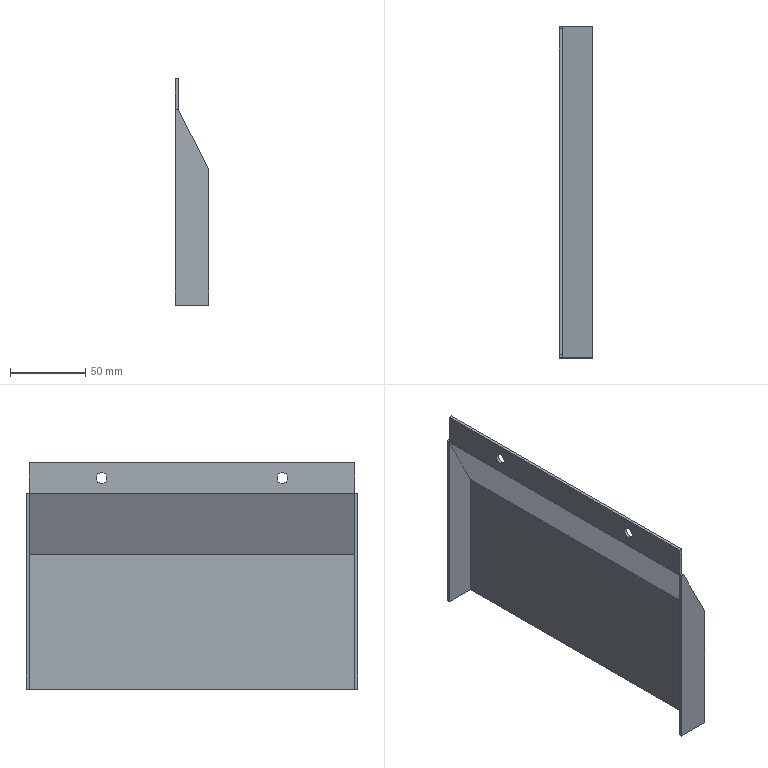Part | SolidWorks | features BaseBody 1 | 1 solid | 20 faces | box 22 x 220 x 150 mm | volume 76517 mm3 | plane 16 | cylinder 4 | commonest cylinder face diameters 7.2 x4
STEP:
#1=CARTESIAN_POINT('',(200.446,-4170.973,253.871));
#2=VERTEX_POINT('',#1);
#3=CARTESIAN_POINT('',(200.446,-4170.973,261.071));
#4=VERTEX_POINT('',#3);
#5=CARTESIAN_POINT('',(200.446,-4170.973,257.471));
#6=DIRECTION('',(-1.,0.,0.));
#7=DIRECTION('',(0.,0.,1.));
#8=AXIS2_PLACEMENT_3D('',#5,#6,#7);
#9=CIRCLE('',#8,3.6);
#10=EDGE_CURVE('',#2,#4,#9,.T.);
#11=ORIENTED_EDGE('',*,*,#10,.F.);
#12=CARTESIAN_POINT('',(198.446,-4170.973,253.871));
#13=VERTEX_POINT('',#12);
#14=CARTESIAN_POINT('',(199.279,-4170.973,253.871));
#15=DIRECTION('',(-1.,0.,0.));
#16=VECTOR('',#15,1000.);
#17=LINE('',#14,#16);
#18=EDGE_CURVE('',#2,#13,#17,.T.);
#19=ORIENTED_EDGE('',*,*,#18,.T.);
#20=CARTESIAN_POINT('',(198.446,-4170.973,261.071));
#21=VERTEX_POINT('',#20);
#22=CARTESIAN_POINT('',(198.446,-4170.973,257.471));
#23=DIRECTION('',(1.,0.,0.));
#24=DIRECTION('',(0.,0.,1.));
#25=AXIS2_PLACEMENT_3D('',#22,#23,#24);
#26=CIRCLE('',#25,3.6);
#27=EDGE_CURVE('',#21,#13,#26,.T.);
#28=ORIENTED_EDGE('',*,*,#27,.F.);
#29=CARTESIAN_POINT('',(199.279,-4170.973,261.071));
#30=DIRECTION('',(-1.,0.,0.));
#31=VECTOR('',#30,1000.);
#32=LINE('',#29,#31);
#33=EDGE_CURVE('',#4,#21,#32,.T.);
#34=ORIENTED_EDGE('',*,*,#33,.F.);
#35=EDGE_LOOP('',(#11,#19,#28,#34));
#36=FACE_OUTER_BOUND('',#35,.T.);
#37=CARTESIAN_POINT('',(199.279,-4170.973,257.471));
#38=DIRECTION('',(-1.,0.,0.));
#39=DIRECTION('',(0.,0.,1.));
#40=AXIS2_PLACEMENT_3D('',#37,#38,#39);
#41=CYLINDRICAL_SURFACE('',#40,3.6);
#42=ADVANCED_FACE('',(#36),#41,.F.);
#43=CARTESIAN_POINT('',(200.446,-4290.973,253.871));
#44=VERTEX_POINT('',#43);
#45=CARTESIAN_POINT('',(200.446,-4290.973,261.071));
#46=VERTEX_POINT('',#45);
#47=CARTESIAN_POINT('',(200.446,-4290.973,257.471));
#48=DIRECTION('',(-1.,0.,0.));
#49=DIRECTION('',(0.,0.,1.));
#50=AXIS2_PLACEMENT_3D('',#47,#48,#49);
#51=CIRCLE('',#50,3.6);
#52=EDGE_CURVE('',#44,#46,#51,.T.);
#53=ORIENTED_EDGE('',*,*,#52,.F.);
#54=CARTESIAN_POINT('',(198.446,-4290.973,253.871));
#55=VERTEX_POINT('',#54);
#56=CARTESIAN_POINT('',(199.279,-4290.973,253.871));
#57=DIRECTION('',(-1.,0.,0.));
#58=VECTOR('',#57,1000.);
#59=LINE('',#56,#58);
#60=EDGE_CURVE('',#44,#55,#59,.T.);
#61=ORIENTED_EDGE('',*,*,#60,.T.);
#62=CARTESIAN_POINT('',(198.446,-4290.973,261.071));
#63=VERTEX_POINT('',#62);
#64=CARTESIAN_POINT('',(198.446,-4290.973,257.471));
#65=DIRECTION('',(1.,0.,0.));
#66=DIRECTION('',(0.,0.,1.));
#67=AXIS2_PLACEMENT_3D('',#64,#65,#66);
#68=CIRCLE('',#67,3.6);
#69=EDGE_CURVE('',#63,#55,#68,.T.);
#70=ORIENTED_EDGE('',*,*,#69,.F.);
#71=CARTESIAN_POINT('',(199.279,-4290.973,261.071));
#72=DIRECTION('',(-1.,0.,0.));
#73=VECTOR('',#72,1000.);
#74=LINE('',#71,#73);
#75=EDGE_CURVE('',#46,#63,#74,.T.);
#76=ORIENTED_EDGE('',*,*,#75,.F.);
#77=EDGE_LOOP('',(#53,#61,#70,#76));
#78=FACE_OUTER_BOUND('',#77,.T.);
#79=CARTESIAN_POINT('',(199.279,-4290.973,257.471));
#80=DIRECTION('',(-1.,0.,0.));
#81=DIRECTION('',(0.,0.,1.));
#82=AXIS2_PLACEMENT_3D('',#79,#80,#81);
#83=CYLINDRICAL_SURFACE('',#82,3.6);
#84=ADVANCED_FACE('',(#78),#83,.F.);
#85=CARTESIAN_POINT('',(220.446,-4120.973,117.471));
#86=VERTEX_POINT('',#85);
#87=CARTESIAN_POINT('',(220.446,-4120.973,207.471));
#88=VERTEX_POINT('',#87);
#89=CARTESIAN_POINT('',(220.446,-4120.973,207.471));
#90=DIRECTION('',(0.,0.,1.));
#91=VECTOR('',#90,1000.);
#92=LINE('',#89,#91);
#93=EDGE_CURVE('',#86,#88,#92,.T.);
#94=ORIENTED_EDGE('',*,*,#93,.T.);
#95=CARTESIAN_POINT('',(220.446,-4340.973,207.471));
#96=VERTEX_POINT('',#95);
#97=CARTESIAN_POINT('',(220.446,-4140.973,207.471));
#98=DIRECTION('',(0.,-1.,0.));
#99=VECTOR('',#98,1000.);
#100=LINE('',#97,#99);
#101=EDGE_CURVE('',#88,#96,#100,.T.);
#102=ORIENTED_EDGE('',*,*,#101,.T.);
#103=CARTESIAN_POINT('',(220.446,-4340.973,117.471));
#104=VERTEX_POINT('',#103);
#105=CARTESIAN_POINT('',(220.446,-4340.973,207.471));
#106=DIRECTION('',(0.,0.,-1.));
#107=VECTOR('',#106,1000.);
#108=LINE('',#105,#107);
#109=EDGE_CURVE('',#96,#104,#108,.T.);
#110=ORIENTED_EDGE('',*,*,#109,.T.);
#111=CARTESIAN_POINT('',(220.446,-4140.973,117.471));
#112=DIRECTION('',(0.,1.,0.));
#113=VECTOR('',#112,1000.);
#114=LINE('',#111,#113);
#115=EDGE_CURVE('',#104,#86,#114,.T.);
#116=ORIENTED_EDGE('',*,*,#115,.T.);
#117=EDGE_LOOP('',(#94,#102,#110,#116));
#118=FACE_OUTER_BOUND('',#117,.T.);
#119=CARTESIAN_POINT('',(220.446,-4140.973,207.471));
#120=DIRECTION('',(1.,0.,0.));
#121=DIRECTION('',(0.,0.,-1.));
#122=AXIS2_PLACEMENT_3D('',#119,#120,#121);
#123=PLANE('',#122);
#124=ADVANCED_FACE('',(#118),#123,.T.);
#125=CARTESIAN_POINT('',(200.446,-4122.973,247.471));
#126=VERTEX_POINT('',#125);
#127=CARTESIAN_POINT('',(200.446,-4338.973,247.471));
#128=VERTEX_POINT('',#127);
#129=CARTESIAN_POINT('',(200.446,-4140.973,247.471));
#130=DIRECTION('',(0.,-1.,0.));
#131=VECTOR('',#130,1000.);
#132=LINE('',#129,#131);
#133=EDGE_CURVE('',#126,#128,#132,.T.);
#134=ORIENTED_EDGE('',*,*,#133,.T.);
#135=CARTESIAN_POINT('',(200.446,-4340.973,247.471));
#136=VERTEX_POINT('',#135);
#137=CARTESIAN_POINT('',(200.446,-4140.973,247.471));
#138=DIRECTION('',(0.,-1.,0.));
#139=VECTOR('',#138,1000.);
#140=LINE('',#137,#139);
#141=EDGE_CURVE('',#128,#136,#140,.T.);
#142=ORIENTED_EDGE('',*,*,#141,.T.);
#143=CARTESIAN_POINT('',(200.446,-4340.973,247.471));
#144=DIRECTION('',(0.4472,0.,-0.8944));
#145=VECTOR('',#144,1000.);
#146=LINE('',#143,#145);
#147=EDGE_CURVE('',#136,#96,#146,.T.);
#148=ORIENTED_EDGE('',*,*,#147,.T.);
#149=ORIENTED_EDGE('',*,*,#101,.F.);
#150=CARTESIAN_POINT('',(200.446,-4120.973,247.471));
#151=VERTEX_POINT('',#150);
#152=CARTESIAN_POINT('',(200.446,-4120.973,247.471));
#153=DIRECTION('',(-0.4472,0.,0.8944));
#154=VECTOR('',#153,1000.);
#155=LINE('',#152,#154);
#156=EDGE_CURVE('',#88,#151,#155,.T.);
#157=ORIENTED_EDGE('',*,*,#156,.T.);
#158=CARTESIAN_POINT('',(200.446,-4140.973,247.471));
#159=DIRECTION('',(0.,-1.,0.));
#160=VECTOR('',#159,1000.);
#161=LINE('',#158,#160);
#162=EDGE_CURVE('',#151,#126,#161,.T.);
#163=ORIENTED_EDGE('',*,*,#162,.T.);
#164=EDGE_LOOP('',(#134,#142,#148,#149,#157,#163));
#165=FACE_OUTER_BOUND('',#164,.T.);
#166=CARTESIAN_POINT('',(200.446,-4140.973,247.471));
#167=DIRECTION('',(0.8944,0.,0.4472));
#168=DIRECTION('',(0.4472,0.,-0.8944));
#169=AXIS2_PLACEMENT_3D('',#166,#167,#168);
#170=PLANE('',#169);
#171=ADVANCED_FACE('',(#165),#170,.T.);
#172=CARTESIAN_POINT('',(198.446,-4120.973,117.471));
#173=VERTEX_POINT('',#172);
#174=CARTESIAN_POINT('',(206.666,-4120.973,117.471));
#175=DIRECTION('',(-1.,0.,0.));
#176=VECTOR('',#175,1000.);
#177=LINE('',#174,#176);
#178=EDGE_CURVE('',#86,#173,#177,.T.);
#179=ORIENTED_EDGE('',*,*,#178,.T.);
#180=CARTESIAN_POINT('',(198.446,-4120.973,247.471));
#181=VERTEX_POINT('',#180);
#182=CARTESIAN_POINT('',(198.446,-4120.973,193.652));
#183=DIRECTION('',(0.,0.,1.));
#184=VECTOR('',#183,1000.);
#185=LINE('',#182,#184);
#186=EDGE_CURVE('',#173,#181,#185,.T.);
#187=ORIENTED_EDGE('',*,*,#186,.T.);
#188=CARTESIAN_POINT('',(206.666,-4120.973,247.471));
#189=DIRECTION('',(1.,0.,0.));
#190=VECTOR('',#189,1000.);
#191=LINE('',#188,#190);
#192=EDGE_CURVE('',#181,#151,#191,.T.);
#193=ORIENTED_EDGE('',*,*,#192,.T.);
#194=ORIENTED_EDGE('',*,*,#156,.F.);
#195=ORIENTED_EDGE('',*,*,#93,.F.);
#196=EDGE_LOOP('',(#179,#187,#193,#194,#195));
#197=FACE_OUTER_BOUND('',#196,.T.);
#198=CARTESIAN_POINT('',(206.666,-4120.973,193.652));
#199=DIRECTION('',(0.,1.,0.));
#200=DIRECTION('',(0.,0.,1.));
#201=AXIS2_PLACEMENT_3D('',#198,#199,#200);
#202=PLANE('',#201);
#203=ADVANCED_FACE('',(#197),#202,.T.);
#204=CARTESIAN_POINT('',(198.446,-4340.973,117.471));
#205=VERTEX_POINT('',#204);
#206=CARTESIAN_POINT('',(218.446,-4340.973,117.471));
#207=DIRECTION('',(-1.,0.,0.));
#208=VECTOR('',#207,1000.);
#209=LINE('',#206,#208);
#210=EDGE_CURVE('',#104,#205,#209,.T.);
#211=ORIENTED_EDGE('',*,*,#210,.T.);
#212=CARTESIAN_POINT('',(198.446,-4338.973,117.471));
#213=VERTEX_POINT('',#212);
#214=CARTESIAN_POINT('',(198.446,-4320.973,117.471));
#215=DIRECTION('',(0.,1.,0.));
#216=VECTOR('',#215,1000.);
#217=LINE('',#214,#216);
#218=EDGE_CURVE('',#205,#213,#217,.T.);
#219=ORIENTED_EDGE('',*,*,#218,.T.);
#220=CARTESIAN_POINT('',(218.446,-4338.973,117.471));
#221=VERTEX_POINT('',#220);
#222=CARTESIAN_POINT('',(218.446,-4338.973,117.471));
#223=DIRECTION('',(1.,0.,0.));
#224=VECTOR('',#223,1000.);
#225=LINE('',#222,#224);
#226=EDGE_CURVE('',#213,#221,#225,.T.);
#227=ORIENTED_EDGE('',*,*,#226,.T.);
#228=CARTESIAN_POINT('',(218.446,-4122.973,117.471));
#229=VERTEX_POINT('',#228);
#230=CARTESIAN_POINT('',(218.446,-4320.973,117.471));
#231=DIRECTION('',(0.,1.,0.));
#232=VECTOR('',#231,1000.);
#233=LINE('',#230,#232);
#234=EDGE_CURVE('',#221,#229,#233,.T.);
#235=ORIENTED_EDGE('',*,*,#234,.T.);
#236=CARTESIAN_POINT('',(198.446,-4122.973,117.471));
#237=VERTEX_POINT('',#236);
#238=CARTESIAN_POINT('',(218.446,-4122.973,117.471));
#239=DIRECTION('',(-1.,0.,0.));
#240=VECTOR('',#239,1000.);
#241=LINE('',#238,#240);
#242=EDGE_CURVE('',#229,#237,#241,.T.);
#243=ORIENTED_EDGE('',*,*,#242,.T.);
#244=CARTESIAN_POINT('',(198.446,-4320.973,117.471));
#245=DIRECTION('',(0.,1.,0.));
#246=VECTOR('',#245,1000.);
#247=LINE('',#244,#246);
#248=EDGE_CURVE('',#237,#173,#247,.T.);
#249=ORIENTED_EDGE('',*,*,#248,.T.);
#250=ORIENTED_EDGE('',*,*,#178,.F.);
#251=ORIENTED_EDGE('',*,*,#115,.F.);
#252=EDGE_LOOP('',(#211,#219,#227,#235,#243,#249,#250,#251));
#253=FACE_OUTER_BOUND('',#252,.T.);
#254=CARTESIAN_POINT('',(218.446,-4320.973,117.471));
#255=DIRECTION('',(0.,0.,-1.));
#256=DIRECTION('',(-1.,0.,0.));
#257=AXIS2_PLACEMENT_3D('',#254,#255,#256);
#258=PLANE('',#257);
#259=ADVANCED_FACE('',(#253),#258,.T.);
#260=ORIENTED_EDGE('',*,*,#109,.F.);
#261=ORIENTED_EDGE('',*,*,#147,.F.);
#262=CARTESIAN_POINT('',(198.446,-4340.973,247.471));
#263=VERTEX_POINT('',#262);
#264=CARTESIAN_POINT('',(206.666,-4340.973,247.471));
#265=DIRECTION('',(-1.,0.,0.));
#266=VECTOR('',#265,1000.);
#267=LINE('',#264,#266);
#268=EDGE_CURVE('',#136,#263,#267,.T.);
#269=ORIENTED_EDGE('',*,*,#268,.T.);
#270=CARTESIAN_POINT('',(198.446,-4340.973,193.652));
#271=DIRECTION('',(0.,0.,-1.));
#272=VECTOR('',#271,1000.);
#273=LINE('',#270,#272);
#274=EDGE_CURVE('',#263,#205,#273,.T.);
#275=ORIENTED_EDGE('',*,*,#274,.T.);
#276=ORIENTED_EDGE('',*,*,#210,.F.);
#277=EDGE_LOOP('',(#260,#261,#269,#275,#276));
#278=FACE_OUTER_BOUND('',#277,.T.);
#279=CARTESIAN_POINT('',(206.666,-4340.973,193.652));
#280=DIRECTION('',(0.,-1.,0.));
#281=DIRECTION('',(0.,0.,-1.));
#282=AXIS2_PLACEMENT_3D('',#279,#280,#281);
#283=PLANE('',#282);
#284=ADVANCED_FACE('',(#278),#283,.T.);
#285=CARTESIAN_POINT('',(198.446,-4338.973,247.471));
#286=VERTEX_POINT('',#285);
#287=CARTESIAN_POINT('',(213.457,-4338.973,247.471));
#288=DIRECTION('',(1.,0.,0.));
#289=VECTOR('',#288,1000.);
#290=LINE('',#287,#289);
#291=EDGE_CURVE('',#286,#128,#290,.T.);
#292=ORIENTED_EDGE('',*,*,#291,.F.);
#293=CARTESIAN_POINT('',(198.446,-4350.722,247.471));
#294=DIRECTION('',(0.,1.,0.));
#295=VECTOR('',#294,1000.);
#296=LINE('',#293,#295);
#297=EDGE_CURVE('',#263,#286,#296,.T.);
#298=ORIENTED_EDGE('',*,*,#297,.F.);
#299=ORIENTED_EDGE('',*,*,#268,.F.);
#300=ORIENTED_EDGE('',*,*,#141,.F.);
#301=EDGE_LOOP('',(#292,#298,#299,#300));
#302=FACE_OUTER_BOUND('',#301,.T.);
#303=CARTESIAN_POINT('',(213.457,-4350.722,247.471));
#304=DIRECTION('',(0.,0.,-1.));
#305=DIRECTION('',(-1.,0.,0.));
#306=AXIS2_PLACEMENT_3D('',#303,#304,#305);
#307=PLANE('',#306);
#308=ADVANCED_FACE('',(#302),#307,.F.);
#309=CARTESIAN_POINT('',(200.446,-4338.973,267.471));
#310=VERTEX_POINT('',#309);
#311=CARTESIAN_POINT('',(200.446,-4338.973,267.471));
#312=DIRECTION('',(0.,0.,-1.));
#313=VECTOR('',#312,1000.);
#314=LINE('',#311,#313);
#315=EDGE_CURVE('',#310,#128,#314,.T.);
#316=ORIENTED_EDGE('',*,*,#315,.T.);
#317=ORIENTED_EDGE('',*,*,#133,.F.);
#318=CARTESIAN_POINT('',(200.446,-4122.973,267.471));
#319=VERTEX_POINT('',#318);
#320=CARTESIAN_POINT('',(200.446,-4122.973,267.471));
#321=DIRECTION('',(0.,0.,1.));
#322=VECTOR('',#321,1000.);
#323=LINE('',#320,#322);
#324=EDGE_CURVE('',#126,#319,#323,.T.);
#325=ORIENTED_EDGE('',*,*,#324,.T.);
#326=CARTESIAN_POINT('',(200.446,-4140.973,267.471));
#327=DIRECTION('',(0.,-1.,0.));
#328=VECTOR('',#327,1000.);
#329=LINE('',#326,#328);
#330=EDGE_CURVE('',#319,#310,#329,.T.);
#331=ORIENTED_EDGE('',*,*,#330,.T.);
#332=EDGE_LOOP('',(#316,#317,#325,#331));
#333=FACE_OUTER_BOUND('',#332,.T.);
#334=CARTESIAN_POINT('',(200.446,-4170.973,257.471));
#335=DIRECTION('',(-1.,0.,0.));
#336=DIRECTION('',(0.,0.,1.));
#337=AXIS2_PLACEMENT_3D('',#334,#335,#336);
#338=CIRCLE('',#337,3.6);
#339=EDGE_CURVE('',#4,#2,#338,.T.);
#340=ORIENTED_EDGE('',*,*,#339,.T.);
#341=ORIENTED_EDGE('',*,*,#10,.T.);
#342=EDGE_LOOP('',(#340,#341));
#343=FACE_BOUND('',#342,.T.);
#344=CARTESIAN_POINT('',(200.446,-4290.973,257.471));
#345=DIRECTION('',(-1.,0.,0.));
#346=DIRECTION('',(0.,0.,1.));
#347=AXIS2_PLACEMENT_3D('',#344,#345,#346);
#348=CIRCLE('',#347,3.6);
#349=EDGE_CURVE('',#46,#44,#348,.T.);
#350=ORIENTED_EDGE('',*,*,#349,.T.);
#351=ORIENTED_EDGE('',*,*,#52,.T.);
#352=EDGE_LOOP('',(#350,#351));
#353=FACE_BOUND('',#352,.T.);
#354=CARTESIAN_POINT('',(200.446,-4140.973,267.471));
#355=DIRECTION('',(1.,0.,0.));
#356=DIRECTION('',(0.,0.,-1.));
#357=AXIS2_PLACEMENT_3D('',#354,#355,#356);
#358=PLANE('',#357);
#359=ADVANCED_FACE('',(#333,#343,#353),#358,.T.);
#360=CARTESIAN_POINT('',(198.446,-4122.973,247.471));
#361=VERTEX_POINT('',#360);
#362=CARTESIAN_POINT('',(213.457,-4122.973,247.471));
#363=DIRECTION('',(-1.,0.,0.));
#364=VECTOR('',#363,1000.);
#365=LINE('',#362,#364);
#366=EDGE_CURVE('',#126,#361,#365,.T.);
#367=ORIENTED_EDGE('',*,*,#366,.F.);
#368=ORIENTED_EDGE('',*,*,#162,.F.);
#369=ORIENTED_EDGE('',*,*,#192,.F.);
#370=CARTESIAN_POINT('',(198.446,-4111.225,247.471));
#371=DIRECTION('',(0.,1.,0.));
#372=VECTOR('',#371,1000.);
#373=LINE('',#370,#372);
#374=EDGE_CURVE('',#361,#181,#373,.T.);
#375=ORIENTED_EDGE('',*,*,#374,.F.);
#376=EDGE_LOOP('',(#367,#368,#369,#375));
#377=FACE_OUTER_BOUND('',#376,.T.);
#378=CARTESIAN_POINT('',(213.457,-4111.225,247.471));
#379=DIRECTION('',(0.,0.,-1.));
#380=DIRECTION('',(-1.,0.,0.));
#381=AXIS2_PLACEMENT_3D('',#378,#379,#380);
#382=PLANE('',#381);
#383=ADVANCED_FACE('',(#377),#382,.F.);
#384=CARTESIAN_POINT('',(198.446,-4338.973,267.471));
#385=VERTEX_POINT('',#384);
#386=CARTESIAN_POINT('',(198.446,-4122.973,267.471));
#387=VERTEX_POINT('',#386);
#388=CARTESIAN_POINT('',(198.446,-4280.973,267.471));
#389=DIRECTION('',(0.,1.,0.));
#390=VECTOR('',#389,1000.);
#391=LINE('',#388,#390);
#392=EDGE_CURVE('',#385,#387,#391,.T.);
#393=ORIENTED_EDGE('',*,*,#392,.T.);
#394=CARTESIAN_POINT('',(198.446,-4122.973,147.471));
#395=DIRECTION('',(0.,0.,-1.));
#396=VECTOR('',#395,1000.);
#397=LINE('',#394,#396);
#398=EDGE_CURVE('',#387,#361,#397,.T.);
#399=ORIENTED_EDGE('',*,*,#398,.T.);
#400=ORIENTED_EDGE('',*,*,#374,.T.);
#401=ORIENTED_EDGE('',*,*,#186,.F.);
#402=ORIENTED_EDGE('',*,*,#248,.F.);
#403=CARTESIAN_POINT('',(198.446,-4122.973,246.999));
#404=VERTEX_POINT('',#403);
#405=CARTESIAN_POINT('',(198.446,-4122.973,147.471));
#406=DIRECTION('',(0.,0.,1.));
#407=VECTOR('',#406,1000.);
#408=LINE('',#405,#407);
#409=EDGE_CURVE('',#237,#404,#408,.T.);
#410=ORIENTED_EDGE('',*,*,#409,.T.);
#411=CARTESIAN_POINT('',(198.446,-4338.973,246.999));
#412=VERTEX_POINT('',#411);
#413=CARTESIAN_POINT('',(198.446,-4280.973,246.999));
#414=DIRECTION('',(0.,-1.,0.));
#415=VECTOR('',#414,1000.);
#416=LINE('',#413,#415);
#417=EDGE_CURVE('',#404,#412,#416,.T.);
#418=ORIENTED_EDGE('',*,*,#417,.T.);
#419=CARTESIAN_POINT('',(198.446,-4338.973,147.471));
#420=DIRECTION('',(0.,0.,-1.));
#421=VECTOR('',#420,1000.);
#422=LINE('',#419,#421);
#423=EDGE_CURVE('',#412,#213,#422,.T.);
#424=ORIENTED_EDGE('',*,*,#423,.T.);
#425=ORIENTED_EDGE('',*,*,#218,.F.);
#426=ORIENTED_EDGE('',*,*,#274,.F.);
#427=ORIENTED_EDGE('',*,*,#297,.T.);
#428=CARTESIAN_POINT('',(198.446,-4338.973,147.471));
#429=DIRECTION('',(0.,0.,1.));
#430=VECTOR('',#429,1000.);
#431=LINE('',#428,#430);
#432=EDGE_CURVE('',#286,#385,#431,.T.);
#433=ORIENTED_EDGE('',*,*,#432,.T.);
#434=EDGE_LOOP('',(#393,#399,#400,#401,#402,#410,#418,#424,#425,#426,#427,#433));
#435=FACE_OUTER_BOUND('',#434,.T.);
#436=ORIENTED_EDGE('',*,*,#27,.T.);
#437=CARTESIAN_POINT('',(198.446,-4170.973,257.471));
#438=DIRECTION('',(1.,0.,0.));
#439=DIRECTION('',(0.,0.,1.));
#440=AXIS2_PLACEMENT_3D('',#437,#438,#439);
#441=CIRCLE('',#440,3.6);
#442=EDGE_CURVE('',#13,#21,#441,.T.);
#443=ORIENTED_EDGE('',*,*,#442,.T.);
#444=EDGE_LOOP('',(#436,#443));
#445=FACE_BOUND('',#444,.T.);
#446=ORIENTED_EDGE('',*,*,#69,.T.);
#447=CARTESIAN_POINT('',(198.446,-4290.973,257.471));
#448=DIRECTION('',(1.,0.,0.));
#449=DIRECTION('',(0.,0.,1.));
#450=AXIS2_PLACEMENT_3D('',#447,#448,#449);
#451=CIRCLE('',#450,3.6);
#452=EDGE_CURVE('',#55,#63,#451,.T.);
#453=ORIENTED_EDGE('',*,*,#452,.T.);
#454=EDGE_LOOP('',(#446,#453));
#455=FACE_BOUND('',#454,.T.);
#456=CARTESIAN_POINT('',(198.446,-4280.973,147.471));
#457=DIRECTION('',(-1.,0.,0.));
#458=DIRECTION('',(0.,0.,1.));
#459=AXIS2_PLACEMENT_3D('',#456,#457,#458);
#460=PLANE('',#459);
#461=ADVANCED_FACE('',(#435,#445,#455),#460,.T.);
#462=ORIENTED_EDGE('',*,*,#409,.F.);
#463=ORIENTED_EDGE('',*,*,#242,.F.);
#464=CARTESIAN_POINT('',(218.446,-4122.973,206.999));
#465=VERTEX_POINT('',#464);
#466=CARTESIAN_POINT('',(218.446,-4122.973,193.652));
#467=DIRECTION('',(0.,0.,-1.));
#468=VECTOR('',#467,1000.);
#469=LINE('',#466,#468);
#470=EDGE_CURVE('',#465,#229,#469,.T.);
#471=ORIENTED_EDGE('',*,*,#470,.F.);
#472=CARTESIAN_POINT('',(198.446,-4122.973,246.999));
#473=DIRECTION('',(0.4472,0.,-0.8944));
#474=VECTOR('',#473,1000.);
#475=LINE('',#472,#474);
#476=EDGE_CURVE('',#404,#465,#475,.T.);
#477=ORIENTED_EDGE('',*,*,#476,.F.);
#478=EDGE_LOOP('',(#462,#463,#471,#477));
#479=FACE_OUTER_BOUND('',#478,.T.);
#480=CARTESIAN_POINT('',(206.666,-4122.973,193.652));
#481=DIRECTION('',(0.,1.,0.));
#482=DIRECTION('',(0.,0.,1.));
#483=AXIS2_PLACEMENT_3D('',#480,#481,#482);
#484=PLANE('',#483);
#485=ADVANCED_FACE('',(#479),#484,.F.);
#486=ORIENTED_EDGE('',*,*,#470,.T.);
#487=ORIENTED_EDGE('',*,*,#234,.F.);
#488=CARTESIAN_POINT('',(218.446,-4338.973,206.999));
#489=VERTEX_POINT('',#488);
#490=CARTESIAN_POINT('',(218.446,-4338.973,117.471));
#491=DIRECTION('',(0.,0.,1.));
#492=VECTOR('',#491,1000.);
#493=LINE('',#490,#492);
#494=EDGE_CURVE('',#221,#489,#493,.T.);
#495=ORIENTED_EDGE('',*,*,#494,.T.);
#496=CARTESIAN_POINT('',(218.446,-4140.973,206.999));
#497=DIRECTION('',(0.,1.,0.));
#498=VECTOR('',#497,1000.);
#499=LINE('',#496,#498);
#500=EDGE_CURVE('',#489,#465,#499,.T.);
#501=ORIENTED_EDGE('',*,*,#500,.T.);
#502=EDGE_LOOP('',(#486,#487,#495,#501));
#503=FACE_OUTER_BOUND('',#502,.T.);
#504=CARTESIAN_POINT('',(218.446,-4140.973,117.471));
#505=DIRECTION('',(-1.,0.,0.));
#506=DIRECTION('',(0.,0.,1.));
#507=AXIS2_PLACEMENT_3D('',#504,#505,#506);
#508=PLANE('',#507);
#509=ADVANCED_FACE('',(#503),#508,.T.);
#510=ORIENTED_EDGE('',*,*,#494,.F.);
#511=ORIENTED_EDGE('',*,*,#226,.F.);
#512=ORIENTED_EDGE('',*,*,#423,.F.);
#513=CARTESIAN_POINT('',(218.446,-4338.973,206.999));
#514=DIRECTION('',(-0.4472,0.,0.8944));
#515=VECTOR('',#514,1000.);
#516=LINE('',#513,#515);
#517=EDGE_CURVE('',#489,#412,#516,.T.);
#518=ORIENTED_EDGE('',*,*,#517,.F.);
#519=EDGE_LOOP('',(#510,#511,#512,#518));
#520=FACE_OUTER_BOUND('',#519,.T.);
#521=CARTESIAN_POINT('',(206.666,-4338.973,193.652));
#522=DIRECTION('',(0.,-1.,0.));
#523=DIRECTION('',(0.,0.,-1.));
#524=AXIS2_PLACEMENT_3D('',#521,#522,#523);
#525=PLANE('',#524);
#526=ADVANCED_FACE('',(#520),#525,.F.);
#527=CARTESIAN_POINT('',(213.457,-4338.973,267.471));
#528=DIRECTION('',(1.,0.,0.));
#529=VECTOR('',#528,1000.);
#530=LINE('',#527,#529);
#531=EDGE_CURVE('',#385,#310,#530,.T.);
#532=ORIENTED_EDGE('',*,*,#531,.F.);
#533=ORIENTED_EDGE('',*,*,#432,.F.);
#534=ORIENTED_EDGE('',*,*,#291,.T.);
#535=ORIENTED_EDGE('',*,*,#315,.F.);
#536=EDGE_LOOP('',(#532,#533,#534,#535));
#537=FACE_OUTER_BOUND('',#536,.T.);
#538=CARTESIAN_POINT('',(213.457,-4338.973,247.471));
#539=DIRECTION('',(0.,1.,0.));
#540=DIRECTION('',(0.,0.,1.));
#541=AXIS2_PLACEMENT_3D('',#538,#539,#540);
#542=PLANE('',#541);
#543=ADVANCED_FACE('',(#537),#542,.F.);
#544=ORIENTED_EDGE('',*,*,#531,.T.);
#545=ORIENTED_EDGE('',*,*,#330,.F.);
#546=CARTESIAN_POINT('',(198.446,-4122.973,267.471));
#547=DIRECTION('',(-1.,0.,0.));
#548=VECTOR('',#547,1000.);
#549=LINE('',#546,#548);
#550=EDGE_CURVE('',#319,#387,#549,.T.);
#551=ORIENTED_EDGE('',*,*,#550,.T.);
#552=ORIENTED_EDGE('',*,*,#392,.F.);
#553=EDGE_LOOP('',(#544,#545,#551,#552));
#554=FACE_OUTER_BOUND('',#553,.T.);
#555=CARTESIAN_POINT('',(198.446,-4140.973,267.471));
#556=DIRECTION('',(0.,0.,1.));
#557=DIRECTION('',(1.,0.,0.));
#558=AXIS2_PLACEMENT_3D('',#555,#556,#557);
#559=PLANE('',#558);
#560=ADVANCED_FACE('',(#554),#559,.T.);
#561=ORIENTED_EDGE('',*,*,#550,.F.);
#562=ORIENTED_EDGE('',*,*,#324,.F.);
#563=ORIENTED_EDGE('',*,*,#366,.T.);
#564=ORIENTED_EDGE('',*,*,#398,.F.);
#565=EDGE_LOOP('',(#561,#562,#563,#564));
#566=FACE_OUTER_BOUND('',#565,.T.);
#567=CARTESIAN_POINT('',(213.457,-4122.973,247.471));
#568=DIRECTION('',(0.,-1.,0.));
#569=DIRECTION('',(0.,0.,-1.));
#570=AXIS2_PLACEMENT_3D('',#567,#568,#569);
#571=PLANE('',#570);
#572=ADVANCED_FACE('',(#566),#571,.F.);
#573=ORIENTED_EDGE('',*,*,#18,.F.);
#574=ORIENTED_EDGE('',*,*,#339,.F.);
#575=ORIENTED_EDGE('',*,*,#33,.T.);
#576=ORIENTED_EDGE('',*,*,#442,.F.);
#577=EDGE_LOOP('',(#573,#574,#575,#576));
#578=FACE_OUTER_BOUND('',#577,.T.);
#579=CARTESIAN_POINT('',(199.279,-4170.973,257.471));
#580=DIRECTION('',(-1.,0.,0.));
#581=DIRECTION('',(0.,0.,1.));
#582=AXIS2_PLACEMENT_3D('',#579,#580,#581);
#583=CYLINDRICAL_SURFACE('',#582,3.6);
#584=ADVANCED_FACE('',(#578),#583,.F.);
#585=ORIENTED_EDGE('',*,*,#60,.F.);
#586=ORIENTED_EDGE('',*,*,#349,.F.);
#587=ORIENTED_EDGE('',*,*,#75,.T.);
#588=ORIENTED_EDGE('',*,*,#452,.F.);
#589=EDGE_LOOP('',(#585,#586,#587,#588));
#590=FACE_OUTER_BOUND('',#589,.T.);
#591=CARTESIAN_POINT('',(199.279,-4290.973,257.471));
#592=DIRECTION('',(-1.,0.,0.));
#593=DIRECTION('',(0.,0.,1.));
#594=AXIS2_PLACEMENT_3D('',#591,#592,#593);
#595=CYLINDRICAL_SURFACE('',#594,3.6);
#596=ADVANCED_FACE('',(#590),#595,.F.);
#597=ORIENTED_EDGE('',*,*,#476,.T.);
#598=ORIENTED_EDGE('',*,*,#500,.F.);
#599=ORIENTED_EDGE('',*,*,#517,.T.);
#600=ORIENTED_EDGE('',*,*,#417,.F.);
#601=EDGE_LOOP('',(#597,#598,#599,#600));
#602=FACE_OUTER_BOUND('',#601,.T.);
#603=CARTESIAN_POINT('',(218.446,-4140.973,206.999));
#604=DIRECTION('',(-0.8944,0.,-0.4472));
#605=DIRECTION('',(-0.4472,0.,0.8944));
#606=AXIS2_PLACEMENT_3D('',#603,#604,#605);
#607=PLANE('',#606);
#608=ADVANCED_FACE('',(#602),#607,.T.);
#609=CLOSED_SHELL('',(#42,#84,#124,#171,#203,#259,#284,#308,#359,#383,#461,#485,#509,#526,#543,#560,#572,#584,#596,#608));
#610=MANIFOLD_SOLID_BREP('',#609);
#611=CARTESIAN_POINT('',(0.,0.,0.));
#612=DIRECTION('',(0.,0.,1.));
#613=DIRECTION('',(1.,0.,0.));
#614=AXIS2_PLACEMENT_3D('',#611,#612,#613);
#615=(LENGTH_UNIT()NAMED_UNIT(*)SI_UNIT(.MILLI.,.METRE.));
#616=UNCERTAINTY_MEASURE_WITH_UNIT(LENGTH_MEASURE(0.00001),#615,'','');
#617=(NAMED_UNIT(*)PLANE_ANGLE_UNIT()SI_UNIT($,.RADIAN.));
#618=(NAMED_UNIT(*)SI_UNIT($,.STERADIAN.)SOLID_ANGLE_UNIT());
#619=(GEOMETRIC_REPRESENTATION_CONTEXT(3)GLOBAL_UNCERTAINTY_ASSIGNED_CONTEXT((#616))GLOBAL_UNIT_ASSIGNED_CONTEXT((#615,#617,#618))REPRESENTATION_CONTEXT('',''));
#620=ADVANCED_BREP_SHAPE_REPRESENTATION('',(#610,#614),#619);